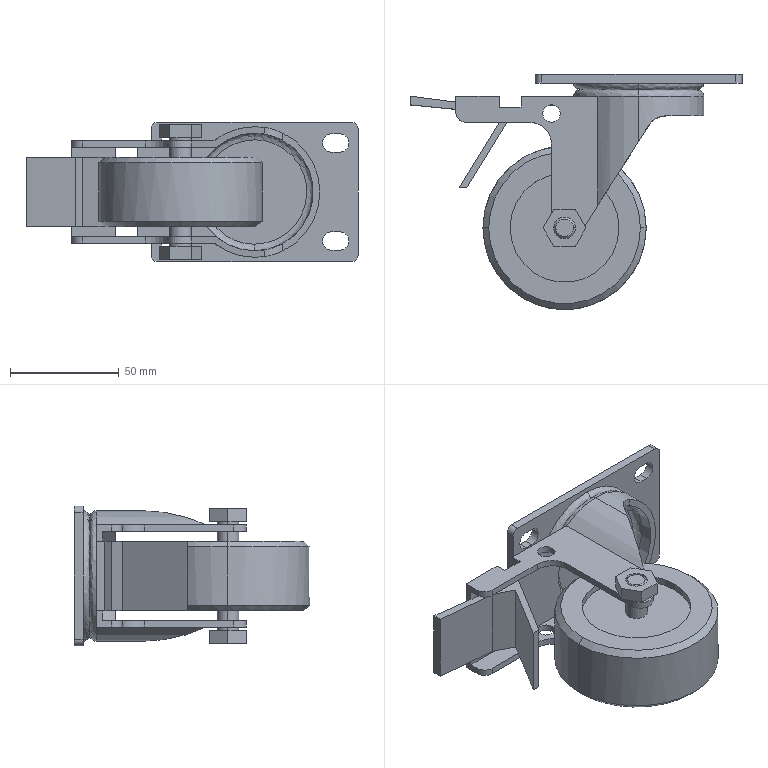Part | SolidWorks | features BaseBody 1 | 1 solid | 134 faces | box 152.5 x 108 x 64 mm | volume 200603 mm3 | plane 70 | cylinder 48 | spline 8 | cone 8 | commonest cylinder face diameters 10 x14 8.5 x8 6 x4 8 x4 20 x4 50 x4